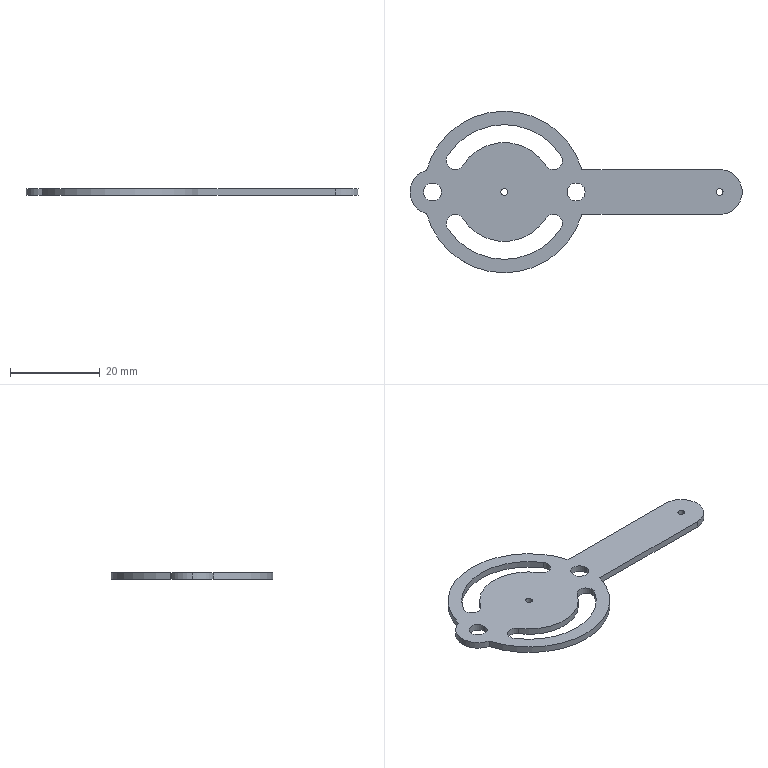Part | SolidWorks | features Extrusion 1 | 1 solid | 27 faces | box 74 x 36 x 1.5 mm | volume 1679 mm3 | cylinder 23 | plane 4 | commonest cylinder face diameters 4 x10 1.5 x4 10 x3 22 x2 30 x2 36 x2
STEP:
#1=CARTESIAN_POINT('',(47.25,0.,1.5));
#2=VERTEX_POINT('',#1);
#3=CARTESIAN_POINT('',(48.75,0.,1.5));
#4=VERTEX_POINT('',#3);
#5=CARTESIAN_POINT('',(48.,0.,1.5));
#6=DIRECTION('',(0.,0.,1.));
#7=DIRECTION('',(1.,0.,0.));
#8=AXIS2_PLACEMENT_3D('',#5,#6,#7);
#9=CIRCLE('',#8,0.75);
#10=EDGE_CURVE('',#2,#4,#9,.T.);
#11=ORIENTED_EDGE('',*,*,#10,.T.);
#12=CARTESIAN_POINT('',(48.75,0.,0.));
#13=VERTEX_POINT('',#12);
#14=CARTESIAN_POINT('',(48.75,0.,1.5));
#15=DIRECTION('',(0.,0.,-1.));
#16=VECTOR('',#15,1000.);
#17=LINE('',#14,#16);
#18=EDGE_CURVE('',#4,#13,#17,.T.);
#19=ORIENTED_EDGE('',*,*,#18,.T.);
#20=CARTESIAN_POINT('',(47.25,0.,0.));
#21=VERTEX_POINT('',#20);
#22=CARTESIAN_POINT('',(48.,0.,0.));
#23=DIRECTION('',(0.,0.,1.));
#24=DIRECTION('',(1.,0.,0.));
#25=AXIS2_PLACEMENT_3D('',#22,#23,#24);
#26=CIRCLE('',#25,0.75);
#27=EDGE_CURVE('',#21,#13,#26,.T.);
#28=ORIENTED_EDGE('',*,*,#27,.F.);
#29=CARTESIAN_POINT('',(47.25,0.,1.5));
#30=DIRECTION('',(0.,0.,-1.));
#31=VECTOR('',#30,1000.);
#32=LINE('',#29,#31);
#33=EDGE_CURVE('',#2,#21,#32,.T.);
#34=ORIENTED_EDGE('',*,*,#33,.F.);
#35=EDGE_LOOP('',(#11,#19,#28,#34));
#36=FACE_OUTER_BOUND('',#35,.T.);
#37=CARTESIAN_POINT('',(48.,0.,1.5));
#38=DIRECTION('',(0.,0.,-1.));
#39=DIRECTION('',(-1.,0.,0.));
#40=AXIS2_PLACEMENT_3D('',#37,#38,#39);
#41=CYLINDRICAL_SURFACE('',#40,0.75);
#42=ADVANCED_FACE('',(#36),#41,.F.);
#43=CARTESIAN_POINT('',(-18.,0.,1.5));
#44=VERTEX_POINT('',#43);
#45=CARTESIAN_POINT('',(-14.,0.,1.5));
#46=VERTEX_POINT('',#45);
#47=CARTESIAN_POINT('',(-16.,0.,1.5));
#48=DIRECTION('',(0.,0.,1.));
#49=DIRECTION('',(1.,0.,0.));
#50=AXIS2_PLACEMENT_3D('',#47,#48,#49);
#51=CIRCLE('',#50,2.);
#52=EDGE_CURVE('',#44,#46,#51,.T.);
#53=ORIENTED_EDGE('',*,*,#52,.T.);
#54=CARTESIAN_POINT('',(-14.,0.,0.));
#55=VERTEX_POINT('',#54);
#56=CARTESIAN_POINT('',(-14.,0.,1.5));
#57=DIRECTION('',(0.,0.,-1.));
#58=VECTOR('',#57,1000.);
#59=LINE('',#56,#58);
#60=EDGE_CURVE('',#46,#55,#59,.T.);
#61=ORIENTED_EDGE('',*,*,#60,.T.);
#62=CARTESIAN_POINT('',(-18.,0.,0.));
#63=VERTEX_POINT('',#62);
#64=CARTESIAN_POINT('',(-16.,0.,0.));
#65=DIRECTION('',(0.,0.,1.));
#66=DIRECTION('',(1.,0.,0.));
#67=AXIS2_PLACEMENT_3D('',#64,#65,#66);
#68=CIRCLE('',#67,2.);
#69=EDGE_CURVE('',#63,#55,#68,.T.);
#70=ORIENTED_EDGE('',*,*,#69,.F.);
#71=CARTESIAN_POINT('',(-18.,0.,1.5));
#72=DIRECTION('',(0.,0.,-1.));
#73=VECTOR('',#72,1000.);
#74=LINE('',#71,#73);
#75=EDGE_CURVE('',#44,#63,#74,.T.);
#76=ORIENTED_EDGE('',*,*,#75,.F.);
#77=EDGE_LOOP('',(#53,#61,#70,#76));
#78=FACE_OUTER_BOUND('',#77,.T.);
#79=CARTESIAN_POINT('',(-16.,0.,1.5));
#80=DIRECTION('',(0.,0.,-1.));
#81=DIRECTION('',(-1.,0.,0.));
#82=AXIS2_PLACEMENT_3D('',#79,#80,#81);
#83=CYLINDRICAL_SURFACE('',#82,2.);
#84=ADVANCED_FACE('',(#78),#83,.F.);
#85=CARTESIAN_POINT('',(14.,0.,1.5));
#86=VERTEX_POINT('',#85);
#87=CARTESIAN_POINT('',(18.,0.,1.5));
#88=VERTEX_POINT('',#87);
#89=CARTESIAN_POINT('',(16.,0.,1.5));
#90=DIRECTION('',(0.,0.,1.));
#91=DIRECTION('',(1.,0.,0.));
#92=AXIS2_PLACEMENT_3D('',#89,#90,#91);
#93=CIRCLE('',#92,2.);
#94=EDGE_CURVE('',#86,#88,#93,.T.);
#95=ORIENTED_EDGE('',*,*,#94,.T.);
#96=CARTESIAN_POINT('',(18.,0.,0.));
#97=VERTEX_POINT('',#96);
#98=CARTESIAN_POINT('',(18.,0.,1.5));
#99=DIRECTION('',(0.,0.,-1.));
#100=VECTOR('',#99,1000.);
#101=LINE('',#98,#100);
#102=EDGE_CURVE('',#88,#97,#101,.T.);
#103=ORIENTED_EDGE('',*,*,#102,.T.);
#104=CARTESIAN_POINT('',(14.,0.,0.));
#105=VERTEX_POINT('',#104);
#106=CARTESIAN_POINT('',(16.,0.,0.));
#107=DIRECTION('',(0.,0.,1.));
#108=DIRECTION('',(1.,0.,0.));
#109=AXIS2_PLACEMENT_3D('',#106,#107,#108);
#110=CIRCLE('',#109,2.);
#111=EDGE_CURVE('',#105,#97,#110,.T.);
#112=ORIENTED_EDGE('',*,*,#111,.F.);
#113=CARTESIAN_POINT('',(14.,0.,1.5));
#114=DIRECTION('',(0.,0.,-1.));
#115=VECTOR('',#114,1000.);
#116=LINE('',#113,#115);
#117=EDGE_CURVE('',#86,#105,#116,.T.);
#118=ORIENTED_EDGE('',*,*,#117,.F.);
#119=EDGE_LOOP('',(#95,#103,#112,#118));
#120=FACE_OUTER_BOUND('',#119,.T.);
#121=CARTESIAN_POINT('',(16.,0.,1.5));
#122=DIRECTION('',(0.,0.,-1.));
#123=DIRECTION('',(-1.,0.,0.));
#124=AXIS2_PLACEMENT_3D('',#121,#122,#123);
#125=CYLINDRICAL_SURFACE('',#124,2.);
#126=ADVANCED_FACE('',(#120),#125,.F.);
#127=CARTESIAN_POINT('',(-9.269,-5.923,1.5));
#128=VERTEX_POINT('',#127);
#129=CARTESIAN_POINT('',(-12.954,-7.,1.5));
#130=VERTEX_POINT('',#129);
#131=CARTESIAN_POINT('',(-10.954,-7.,1.5));
#132=DIRECTION('',(0.,0.,1.));
#133=DIRECTION('',(1.,0.,0.));
#134=AXIS2_PLACEMENT_3D('',#131,#132,#133);
#135=CIRCLE('',#134,2.);
#136=EDGE_CURVE('',#128,#130,#135,.T.);
#137=ORIENTED_EDGE('',*,*,#136,.T.);
#138=CARTESIAN_POINT('',(-12.954,-7.,0.));
#139=VERTEX_POINT('',#138);
#140=CARTESIAN_POINT('',(-12.954,-7.,1.5));
#141=DIRECTION('',(0.,0.,-1.));
#142=VECTOR('',#141,1000.);
#143=LINE('',#140,#142);
#144=EDGE_CURVE('',#130,#139,#143,.T.);
#145=ORIENTED_EDGE('',*,*,#144,.T.);
#146=CARTESIAN_POINT('',(-9.269,-5.923,0.));
#147=VERTEX_POINT('',#146);
#148=CARTESIAN_POINT('',(-10.954,-7.,0.));
#149=DIRECTION('',(0.,0.,1.));
#150=DIRECTION('',(1.,0.,0.));
#151=AXIS2_PLACEMENT_3D('',#148,#149,#150);
#152=CIRCLE('',#151,2.);
#153=EDGE_CURVE('',#147,#139,#152,.T.);
#154=ORIENTED_EDGE('',*,*,#153,.F.);
#155=CARTESIAN_POINT('',(-9.269,-5.923,1.5));
#156=DIRECTION('',(0.,0.,-1.));
#157=VECTOR('',#156,1000.);
#158=LINE('',#155,#157);
#159=EDGE_CURVE('',#128,#147,#158,.T.);
#160=ORIENTED_EDGE('',*,*,#159,.F.);
#161=EDGE_LOOP('',(#137,#145,#154,#160));
#162=FACE_OUTER_BOUND('',#161,.T.);
#163=CARTESIAN_POINT('',(-10.954,-7.,1.5));
#164=DIRECTION('',(0.,0.,-1.));
#165=DIRECTION('',(-1.,0.,0.));
#166=AXIS2_PLACEMENT_3D('',#163,#164,#165);
#167=CYLINDRICAL_SURFACE('',#166,2.);
#168=ADVANCED_FACE('',(#162),#167,.F.);
#169=CARTESIAN_POINT('',(-0.75,0.,1.5));
#170=VERTEX_POINT('',#169);
#171=CARTESIAN_POINT('',(0.75,0.,1.5));
#172=VERTEX_POINT('',#171);
#173=CARTESIAN_POINT('',(0.,0.,1.5));
#174=DIRECTION('',(0.,0.,1.));
#175=DIRECTION('',(1.,0.,0.));
#176=AXIS2_PLACEMENT_3D('',#173,#174,#175);
#177=CIRCLE('',#176,0.75);
#178=EDGE_CURVE('',#170,#172,#177,.T.);
#179=ORIENTED_EDGE('',*,*,#178,.T.);
#180=CARTESIAN_POINT('',(0.75,0.,0.));
#181=VERTEX_POINT('',#180);
#182=CARTESIAN_POINT('',(0.75,0.,1.5));
#183=DIRECTION('',(0.,0.,-1.));
#184=VECTOR('',#183,1000.);
#185=LINE('',#182,#184);
#186=EDGE_CURVE('',#172,#181,#185,.T.);
#187=ORIENTED_EDGE('',*,*,#186,.T.);
#188=CARTESIAN_POINT('',(-0.75,0.,0.));
#189=VERTEX_POINT('',#188);
#190=CARTESIAN_POINT('',(0.,0.,0.));
#191=DIRECTION('',(0.,0.,1.));
#192=DIRECTION('',(1.,0.,0.));
#193=AXIS2_PLACEMENT_3D('',#190,#191,#192);
#194=CIRCLE('',#193,0.75);
#195=EDGE_CURVE('',#189,#181,#194,.T.);
#196=ORIENTED_EDGE('',*,*,#195,.F.);
#197=CARTESIAN_POINT('',(-0.75,0.,1.5));
#198=DIRECTION('',(0.,0.,-1.));
#199=VECTOR('',#198,1000.);
#200=LINE('',#197,#199);
#201=EDGE_CURVE('',#170,#189,#200,.T.);
#202=ORIENTED_EDGE('',*,*,#201,.F.);
#203=EDGE_LOOP('',(#179,#187,#196,#202));
#204=FACE_OUTER_BOUND('',#203,.T.);
#205=CARTESIAN_POINT('',(0.,0.,1.5));
#206=DIRECTION('',(0.,0.,-1.));
#207=DIRECTION('',(-1.,0.,0.));
#208=AXIS2_PLACEMENT_3D('',#205,#206,#207);
#209=CYLINDRICAL_SURFACE('',#208,0.75);
#210=ADVANCED_FACE('',(#204),#209,.F.);
#211=CARTESIAN_POINT('',(-12.64,8.077,1.5));
#212=VERTEX_POINT('',#211);
#213=CARTESIAN_POINT('',(-12.954,7.,1.5));
#214=VERTEX_POINT('',#213);
#215=CARTESIAN_POINT('',(-10.954,7.,1.5));
#216=DIRECTION('',(0.,0.,1.));
#217=DIRECTION('',(1.,0.,0.));
#218=AXIS2_PLACEMENT_3D('',#215,#216,#217);
#219=CIRCLE('',#218,2.);
#220=EDGE_CURVE('',#212,#214,#219,.T.);
#221=ORIENTED_EDGE('',*,*,#220,.T.);
#222=CARTESIAN_POINT('',(-12.954,7.,0.));
#223=VERTEX_POINT('',#222);
#224=CARTESIAN_POINT('',(-12.954,7.,1.5));
#225=DIRECTION('',(0.,0.,-1.));
#226=VECTOR('',#225,1000.);
#227=LINE('',#224,#226);
#228=EDGE_CURVE('',#214,#223,#227,.T.);
#229=ORIENTED_EDGE('',*,*,#228,.T.);
#230=CARTESIAN_POINT('',(-12.64,8.077,0.));
#231=VERTEX_POINT('',#230);
#232=CARTESIAN_POINT('',(-10.954,7.,0.));
#233=DIRECTION('',(0.,0.,1.));
#234=DIRECTION('',(1.,0.,0.));
#235=AXIS2_PLACEMENT_3D('',#232,#233,#234);
#236=CIRCLE('',#235,2.);
#237=EDGE_CURVE('',#231,#223,#236,.T.);
#238=ORIENTED_EDGE('',*,*,#237,.F.);
#239=CARTESIAN_POINT('',(-12.64,8.077,1.5));
#240=DIRECTION('',(0.,0.,-1.));
#241=VECTOR('',#240,1000.);
#242=LINE('',#239,#241);
#243=EDGE_CURVE('',#212,#231,#242,.T.);
#244=ORIENTED_EDGE('',*,*,#243,.F.);
#245=EDGE_LOOP('',(#221,#229,#238,#244));
#246=FACE_OUTER_BOUND('',#245,.T.);
#247=CARTESIAN_POINT('',(-10.954,7.,1.5));
#248=DIRECTION('',(0.,0.,-1.));
#249=DIRECTION('',(-1.,0.,0.));
#250=AXIS2_PLACEMENT_3D('',#247,#248,#249);
#251=CYLINDRICAL_SURFACE('',#250,2.);
#252=ADVANCED_FACE('',(#246),#251,.F.);
#253=CARTESIAN_POINT('',(-21.,0.,1.5));
#254=VERTEX_POINT('',#253);
#255=CARTESIAN_POINT('',(-17.344,-4.816,1.5));
#256=VERTEX_POINT('',#255);
#257=CARTESIAN_POINT('',(-16.,0.,1.5));
#258=DIRECTION('',(0.,0.,1.));
#259=DIRECTION('',(1.,0.,0.));
#260=AXIS2_PLACEMENT_3D('',#257,#258,#259);
#261=CIRCLE('',#260,5.);
#262=EDGE_CURVE('',#254,#256,#261,.T.);
#263=ORIENTED_EDGE('',*,*,#262,.F.);
#264=CARTESIAN_POINT('',(-21.,0.,0.));
#265=VERTEX_POINT('',#264);
#266=CARTESIAN_POINT('',(-21.,0.,1.5));
#267=DIRECTION('',(0.,0.,-1.));
#268=VECTOR('',#267,1000.);
#269=LINE('',#266,#268);
#270=EDGE_CURVE('',#254,#265,#269,.T.);
#271=ORIENTED_EDGE('',*,*,#270,.T.);
#272=CARTESIAN_POINT('',(-17.344,-4.816,0.));
#273=VERTEX_POINT('',#272);
#274=CARTESIAN_POINT('',(-16.,0.,0.));
#275=DIRECTION('',(0.,0.,1.));
#276=DIRECTION('',(1.,0.,0.));
#277=AXIS2_PLACEMENT_3D('',#274,#275,#276);
#278=CIRCLE('',#277,5.);
#279=EDGE_CURVE('',#265,#273,#278,.T.);
#280=ORIENTED_EDGE('',*,*,#279,.T.);
#281=CARTESIAN_POINT('',(-17.344,-4.816,1.5));
#282=DIRECTION('',(0.,0.,-1.));
#283=VECTOR('',#282,1000.);
#284=LINE('',#281,#283);
#285=EDGE_CURVE('',#256,#273,#284,.T.);
#286=ORIENTED_EDGE('',*,*,#285,.F.);
#287=EDGE_LOOP('',(#263,#271,#280,#286));
#288=FACE_OUTER_BOUND('',#287,.T.);
#289=CARTESIAN_POINT('',(-16.,0.,1.5));
#290=DIRECTION('',(0.,0.,-1.));
#291=DIRECTION('',(-1.,0.,0.));
#292=AXIS2_PLACEMENT_3D('',#289,#290,#291);
#293=CYLINDRICAL_SURFACE('',#292,5.);
#294=ADVANCED_FACE('',(#288),#293,.T.);
#295=ORIENTED_EDGE('',*,*,#52,.F.);
#296=CARTESIAN_POINT('',(-16.,0.,1.5));
#297=DIRECTION('',(0.,0.,1.));
#298=DIRECTION('',(1.,0.,0.));
#299=AXIS2_PLACEMENT_3D('',#296,#297,#298);
#300=CIRCLE('',#299,2.);
#301=EDGE_CURVE('',#46,#44,#300,.T.);
#302=ORIENTED_EDGE('',*,*,#301,.F.);
#303=EDGE_LOOP('',(#295,#302));
#304=FACE_BOUND('',#303,.T.);
#305=ORIENTED_EDGE('',*,*,#136,.F.);
#306=CARTESIAN_POINT('',(9.269,-5.923,1.5));
#307=VERTEX_POINT('',#306);
#308=CARTESIAN_POINT('',(0.,0.,1.5));
#309=DIRECTION('',(0.,0.,-1.));
#310=DIRECTION('',(1.,0.,0.));
#311=AXIS2_PLACEMENT_3D('',#308,#309,#310);
#312=CIRCLE('',#311,11.);
#313=EDGE_CURVE('',#307,#128,#312,.T.);
#314=ORIENTED_EDGE('',*,*,#313,.F.);
#315=CARTESIAN_POINT('',(12.64,-8.077,1.5));
#316=VERTEX_POINT('',#315);
#317=CARTESIAN_POINT('',(10.954,-7.,1.5));
#318=DIRECTION('',(0.,0.,1.));
#319=DIRECTION('',(1.,0.,0.));
#320=AXIS2_PLACEMENT_3D('',#317,#318,#319);
#321=CIRCLE('',#320,2.);
#322=EDGE_CURVE('',#316,#307,#321,.T.);
#323=ORIENTED_EDGE('',*,*,#322,.F.);
#324=CARTESIAN_POINT('',(-12.64,-8.077,1.5));
#325=VERTEX_POINT('',#324);
#326=CARTESIAN_POINT('',(0.,0.,1.5));
#327=DIRECTION('',(0.,0.,1.));
#328=DIRECTION('',(1.,0.,0.));
#329=AXIS2_PLACEMENT_3D('',#326,#327,#328);
#330=CIRCLE('',#329,15.);
#331=EDGE_CURVE('',#325,#316,#330,.T.);
#332=ORIENTED_EDGE('',*,*,#331,.F.);
#333=CARTESIAN_POINT('',(-10.954,-7.,1.5));
#334=DIRECTION('',(0.,0.,1.));
#335=DIRECTION('',(1.,0.,0.));
#336=AXIS2_PLACEMENT_3D('',#333,#334,#335);
#337=CIRCLE('',#336,2.);
#338=EDGE_CURVE('',#130,#325,#337,.T.);
#339=ORIENTED_EDGE('',*,*,#338,.F.);
#340=EDGE_LOOP('',(#305,#314,#323,#332,#339));
#341=FACE_BOUND('',#340,.T.);
#342=ORIENTED_EDGE('',*,*,#178,.F.);
#343=CARTESIAN_POINT('',(0.,0.,1.5));
#344=DIRECTION('',(0.,0.,1.));
#345=DIRECTION('',(1.,0.,0.));
#346=AXIS2_PLACEMENT_3D('',#343,#344,#345);
#347=CIRCLE('',#346,0.75);
#348=EDGE_CURVE('',#172,#170,#347,.T.);
#349=ORIENTED_EDGE('',*,*,#348,.F.);
#350=EDGE_LOOP('',(#342,#349));
#351=FACE_BOUND('',#350,.T.);
#352=CARTESIAN_POINT('',(-17.344,4.816,1.5));
#353=VERTEX_POINT('',#352);
#354=CARTESIAN_POINT('',(-16.,0.,1.5));
#355=DIRECTION('',(0.,0.,1.));
#356=DIRECTION('',(1.,0.,0.));
#357=AXIS2_PLACEMENT_3D('',#354,#355,#356);
#358=CIRCLE('',#357,5.);
#359=EDGE_CURVE('',#353,#254,#358,.T.);
#360=ORIENTED_EDGE('',*,*,#359,.T.);
#361=ORIENTED_EDGE('',*,*,#262,.T.);
#362=CARTESIAN_POINT('',(17.292,-5.,1.5));
#363=VERTEX_POINT('',#362);
#364=CARTESIAN_POINT('',(0.,0.,1.5));
#365=DIRECTION('',(0.,0.,1.));
#366=DIRECTION('',(1.,0.,0.));
#367=AXIS2_PLACEMENT_3D('',#364,#365,#366);
#368=CIRCLE('',#367,18.);
#369=EDGE_CURVE('',#256,#363,#368,.T.);
#370=ORIENTED_EDGE('',*,*,#369,.T.);
#371=CARTESIAN_POINT('',(48.,-5.,1.5));
#372=VERTEX_POINT('',#371);
#373=CARTESIAN_POINT('',(48.,-5.,1.5));
#374=DIRECTION('',(1.,0.,0.));
#375=VECTOR('',#374,1000.);
#376=LINE('',#373,#375);
#377=EDGE_CURVE('',#363,#372,#376,.T.);
#378=ORIENTED_EDGE('',*,*,#377,.T.);
#379=CARTESIAN_POINT('',(48.,5.,1.5));
#380=VERTEX_POINT('',#379);
#381=CARTESIAN_POINT('',(48.,0.,1.5));
#382=DIRECTION('',(0.,0.,1.));
#383=DIRECTION('',(-1.,0.,0.));
#384=AXIS2_PLACEMENT_3D('',#381,#382,#383);
#385=CIRCLE('',#384,5.);
#386=EDGE_CURVE('',#372,#380,#385,.T.);
#387=ORIENTED_EDGE('',*,*,#386,.T.);
#388=CARTESIAN_POINT('',(17.292,5.,1.5));
#389=VERTEX_POINT('',#388);
#390=CARTESIAN_POINT('',(48.,5.,1.5));
#391=DIRECTION('',(-1.,0.,0.));
#392=VECTOR('',#391,1000.);
#393=LINE('',#390,#392);
#394=EDGE_CURVE('',#380,#389,#393,.T.);
#395=ORIENTED_EDGE('',*,*,#394,.T.);
#396=CARTESIAN_POINT('',(0.,0.,1.5));
#397=DIRECTION('',(0.,0.,1.));
#398=DIRECTION('',(1.,0.,0.));
#399=AXIS2_PLACEMENT_3D('',#396,#397,#398);
#400=CIRCLE('',#399,18.);
#401=EDGE_CURVE('',#389,#353,#400,.T.);
#402=ORIENTED_EDGE('',*,*,#401,.T.);
#403=EDGE_LOOP('',(#360,#361,#370,#378,#387,#395,#402));
#404=FACE_OUTER_BOUND('',#403,.T.);
#405=ORIENTED_EDGE('',*,*,#220,.F.);
#406=CARTESIAN_POINT('',(12.64,8.077,1.5));
#407=VERTEX_POINT('',#406);
#408=CARTESIAN_POINT('',(0.,0.,1.5));
#409=DIRECTION('',(0.,0.,1.));
#410=DIRECTION('',(1.,0.,0.));
#411=AXIS2_PLACEMENT_3D('',#408,#409,#410);
#412=CIRCLE('',#411,15.);
#413=EDGE_CURVE('',#407,#212,#412,.T.);
#414=ORIENTED_EDGE('',*,*,#413,.F.);
#415=CARTESIAN_POINT('',(9.269,5.923,1.5));
#416=VERTEX_POINT('',#415);
#417=CARTESIAN_POINT('',(10.954,7.,1.5));
#418=DIRECTION('',(0.,0.,1.));
#419=DIRECTION('',(1.,0.,0.));
#420=AXIS2_PLACEMENT_3D('',#417,#418,#419);
#421=CIRCLE('',#420,2.);
#422=EDGE_CURVE('',#416,#407,#421,.T.);
#423=ORIENTED_EDGE('',*,*,#422,.F.);
#424=CARTESIAN_POINT('',(-9.269,5.923,1.5));
#425=VERTEX_POINT('',#424);
#426=CARTESIAN_POINT('',(0.,0.,1.5));
#427=DIRECTION('',(0.,0.,-1.));
#428=DIRECTION('',(1.,0.,0.));
#429=AXIS2_PLACEMENT_3D('',#426,#427,#428);
#430=CIRCLE('',#429,11.);
#431=EDGE_CURVE('',#425,#416,#430,.T.);
#432=ORIENTED_EDGE('',*,*,#431,.F.);
#433=CARTESIAN_POINT('',(-10.954,7.,1.5));
#434=DIRECTION('',(0.,0.,1.));
#435=DIRECTION('',(1.,0.,0.));
#436=AXIS2_PLACEMENT_3D('',#433,#434,#435);
#437=CIRCLE('',#436,2.);
#438=EDGE_CURVE('',#214,#425,#437,.T.);
#439=ORIENTED_EDGE('',*,*,#438,.F.);
#440=EDGE_LOOP('',(#405,#414,#423,#432,#439));
#441=FACE_BOUND('',#440,.T.);
#442=ORIENTED_EDGE('',*,*,#94,.F.);
#443=CARTESIAN_POINT('',(16.,0.,1.5));
#444=DIRECTION('',(0.,0.,1.));
#445=DIRECTION('',(1.,0.,0.));
#446=AXIS2_PLACEMENT_3D('',#443,#444,#445);
#447=CIRCLE('',#446,2.);
#448=EDGE_CURVE('',#88,#86,#447,.T.);
#449=ORIENTED_EDGE('',*,*,#448,.F.);
#450=EDGE_LOOP('',(#442,#449));
#451=FACE_BOUND('',#450,.T.);
#452=ORIENTED_EDGE('',*,*,#10,.F.);
#453=CARTESIAN_POINT('',(48.,0.,1.5));
#454=DIRECTION('',(0.,0.,1.));
#455=DIRECTION('',(1.,0.,0.));
#456=AXIS2_PLACEMENT_3D('',#453,#454,#455);
#457=CIRCLE('',#456,0.75);
#458=EDGE_CURVE('',#4,#2,#457,.T.);
#459=ORIENTED_EDGE('',*,*,#458,.F.);
#460=EDGE_LOOP('',(#452,#459));
#461=FACE_BOUND('',#460,.T.);
#462=CARTESIAN_POINT('',(-16.,0.,1.5));
#463=DIRECTION('',(0.,0.,1.));
#464=DIRECTION('',(1.,0.,0.));
#465=AXIS2_PLACEMENT_3D('',#462,#463,#464);
#466=PLANE('',#465);
#467=ADVANCED_FACE('',(#304,#341,#351,#404,#441,#451,#461),#466,.T.);
#468=ORIENTED_EDGE('',*,*,#195,.T.);
#469=CARTESIAN_POINT('',(0.,0.,0.));
#470=DIRECTION('',(0.,0.,1.));
#471=DIRECTION('',(1.,0.,0.));
#472=AXIS2_PLACEMENT_3D('',#469,#470,#471);
#473=CIRCLE('',#472,0.75);
#474=EDGE_CURVE('',#181,#189,#473,.T.);
#475=ORIENTED_EDGE('',*,*,#474,.T.);
#476=EDGE_LOOP('',(#468,#475));
#477=FACE_BOUND('',#476,.T.);
#478=CARTESIAN_POINT('',(12.64,8.077,0.));
#479=VERTEX_POINT('',#478);
#480=CARTESIAN_POINT('',(0.,0.,0.));
#481=DIRECTION('',(0.,0.,1.));
#482=DIRECTION('',(1.,0.,0.));
#483=AXIS2_PLACEMENT_3D('',#480,#481,#482);
#484=CIRCLE('',#483,15.);
#485=EDGE_CURVE('',#479,#231,#484,.T.);
#486=ORIENTED_EDGE('',*,*,#485,.T.);
#487=ORIENTED_EDGE('',*,*,#237,.T.);
#488=CARTESIAN_POINT('',(-9.269,5.923,0.));
#489=VERTEX_POINT('',#488);
#490=CARTESIAN_POINT('',(-10.954,7.,0.));
#491=DIRECTION('',(0.,0.,1.));
#492=DIRECTION('',(1.,0.,0.));
#493=AXIS2_PLACEMENT_3D('',#490,#491,#492);
#494=CIRCLE('',#493,2.);
#495=EDGE_CURVE('',#223,#489,#494,.T.);
#496=ORIENTED_EDGE('',*,*,#495,.T.);
#497=CARTESIAN_POINT('',(9.269,5.923,0.));
#498=VERTEX_POINT('',#497);
#499=CARTESIAN_POINT('',(0.,0.,0.));
#500=DIRECTION('',(0.,0.,-1.));
#501=DIRECTION('',(1.,0.,0.));
#502=AXIS2_PLACEMENT_3D('',#499,#500,#501);
#503=CIRCLE('',#502,11.);
#504=EDGE_CURVE('',#489,#498,#503,.T.);
#505=ORIENTED_EDGE('',*,*,#504,.T.);
#506=CARTESIAN_POINT('',(10.954,7.,0.));
#507=DIRECTION('',(0.,0.,1.));
#508=DIRECTION('',(1.,0.,0.));
#509=AXIS2_PLACEMENT_3D('',#506,#507,#508);
#510=CIRCLE('',#509,2.);
#511=EDGE_CURVE('',#498,#479,#510,.T.);
#512=ORIENTED_EDGE('',*,*,#511,.T.);
#513=EDGE_LOOP('',(#486,#487,#496,#505,#512));
#514=FACE_BOUND('',#513,.T.);
#515=CARTESIAN_POINT('',(-17.344,4.816,0.));
#516=VERTEX_POINT('',#515);
#517=CARTESIAN_POINT('',(-16.,0.,0.));
#518=DIRECTION('',(0.,0.,1.));
#519=DIRECTION('',(1.,0.,0.));
#520=AXIS2_PLACEMENT_3D('',#517,#518,#519);
#521=CIRCLE('',#520,5.);
#522=EDGE_CURVE('',#516,#265,#521,.T.);
#523=ORIENTED_EDGE('',*,*,#522,.F.);
#524=CARTESIAN_POINT('',(17.292,5.,0.));
#525=VERTEX_POINT('',#524);
#526=CARTESIAN_POINT('',(0.,0.,0.));
#527=DIRECTION('',(0.,0.,1.));
#528=DIRECTION('',(1.,0.,0.));
#529=AXIS2_PLACEMENT_3D('',#526,#527,#528);
#530=CIRCLE('',#529,18.);
#531=EDGE_CURVE('',#525,#516,#530,.T.);
#532=ORIENTED_EDGE('',*,*,#531,.F.);
#533=CARTESIAN_POINT('',(48.,5.,0.));
#534=VERTEX_POINT('',#533);
#535=CARTESIAN_POINT('',(48.,5.,0.));
#536=DIRECTION('',(-1.,0.,0.));
#537=VECTOR('',#536,1000.);
#538=LINE('',#535,#537);
#539=EDGE_CURVE('',#534,#525,#538,.T.);
#540=ORIENTED_EDGE('',*,*,#539,.F.);
#541=CARTESIAN_POINT('',(48.,-5.,0.));
#542=VERTEX_POINT('',#541);
#543=CARTESIAN_POINT('',(48.,0.,0.));
#544=DIRECTION('',(0.,0.,1.));
#545=DIRECTION('',(-1.,0.,0.));
#546=AXIS2_PLACEMENT_3D('',#543,#544,#545);
#547=CIRCLE('',#546,5.);
#548=EDGE_CURVE('',#542,#534,#547,.T.);
#549=ORIENTED_EDGE('',*,*,#548,.F.);
#550=CARTESIAN_POINT('',(17.292,-5.,0.));
#551=VERTEX_POINT('',#550);
#552=CARTESIAN_POINT('',(48.,-5.,0.));
#553=DIRECTION('',(1.,0.,0.));
#554=VECTOR('',#553,1000.);
#555=LINE('',#552,#554);
#556=EDGE_CURVE('',#551,#542,#555,.T.);
#557=ORIENTED_EDGE('',*,*,#556,.F.);
#558=CARTESIAN_POINT('',(0.,0.,0.));
#559=DIRECTION('',(0.,0.,1.));
#560=DIRECTION('',(1.,0.,0.));
#561=AXIS2_PLACEMENT_3D('',#558,#559,#560);
#562=CIRCLE('',#561,18.);
#563=EDGE_CURVE('',#273,#551,#562,.T.);
#564=ORIENTED_EDGE('',*,*,#563,.F.);
#565=ORIENTED_EDGE('',*,*,#279,.F.);
#566=EDGE_LOOP('',(#523,#532,#540,#549,#557,#564,#565));
#567=FACE_OUTER_BOUND('',#566,.T.);
#568=CARTESIAN_POINT('',(9.269,-5.923,0.));
#569=VERTEX_POINT('',#568);
#570=CARTESIAN_POINT('',(0.,0.,0.));
#571=DIRECTION('',(0.,0.,-1.));
#572=DIRECTION('',(1.,0.,0.));
#573=AXIS2_PLACEMENT_3D('',#570,#571,#572);
#574=CIRCLE('',#573,11.);
#575=EDGE_CURVE('',#569,#147,#574,.T.);
#576=ORIENTED_EDGE('',*,*,#575,.T.);
#577=ORIENTED_EDGE('',*,*,#153,.T.);
#578=CARTESIAN_POINT('',(-12.64,-8.077,0.));
#579=VERTEX_POINT('',#578);
#580=CARTESIAN_POINT('',(-10.954,-7.,0.));
#581=DIRECTION('',(0.,0.,1.));
#582=DIRECTION('',(1.,0.,0.));
#583=AXIS2_PLACEMENT_3D('',#580,#581,#582);
#584=CIRCLE('',#583,2.);
#585=EDGE_CURVE('',#139,#579,#584,.T.);
#586=ORIENTED_EDGE('',*,*,#585,.T.);
#587=CARTESIAN_POINT('',(12.64,-8.077,0.));
#588=VERTEX_POINT('',#587);
#589=CARTESIAN_POINT('',(0.,0.,0.));
#590=DIRECTION('',(0.,0.,1.));
#591=DIRECTION('',(1.,0.,0.));
#592=AXIS2_PLACEMENT_3D('',#589,#590,#591);
#593=CIRCLE('',#592,15.);
#594=EDGE_CURVE('',#579,#588,#593,.T.);
#595=ORIENTED_EDGE('',*,*,#594,.T.);
#596=CARTESIAN_POINT('',(10.954,-7.,0.));
#597=DIRECTION('',(0.,0.,1.));
#598=DIRECTION('',(1.,0.,0.));
#599=AXIS2_PLACEMENT_3D('',#596,#597,#598);
#600=CIRCLE('',#599,2.);
#601=EDGE_CURVE('',#588,#569,#600,.T.);
#602=ORIENTED_EDGE('',*,*,#601,.T.);
#603=EDGE_LOOP('',(#576,#577,#586,#595,#602));
#604=FACE_BOUND('',#603,.T.);
#605=ORIENTED_EDGE('',*,*,#111,.T.);
#606=CARTESIAN_POINT('',(16.,0.,0.));
#607=DIRECTION('',(0.,0.,1.));
#608=DIRECTION('',(1.,0.,0.));
#609=AXIS2_PLACEMENT_3D('',#606,#607,#608);
#610=CIRCLE('',#609,2.);
#611=EDGE_CURVE('',#97,#105,#610,.T.);
#612=ORIENTED_EDGE('',*,*,#611,.T.);
#613=EDGE_LOOP('',(#605,#612));
#614=FACE_BOUND('',#613,.T.);
#615=ORIENTED_EDGE('',*,*,#69,.T.);
#616=CARTESIAN_POINT('',(-16.,0.,0.));
#617=DIRECTION('',(0.,0.,1.));
#618=DIRECTION('',(1.,0.,0.));
#619=AXIS2_PLACEMENT_3D('',#616,#617,#618);
#620=CIRCLE('',#619,2.);
#621=EDGE_CURVE('',#55,#63,#620,.T.);
#622=ORIENTED_EDGE('',*,*,#621,.T.);
#623=EDGE_LOOP('',(#615,#622));
#624=FACE_BOUND('',#623,.T.);
#625=ORIENTED_EDGE('',*,*,#27,.T.);
#626=CARTESIAN_POINT('',(48.,0.,0.));
#627=DIRECTION('',(0.,0.,1.));
#628=DIRECTION('',(1.,0.,0.));
#629=AXIS2_PLACEMENT_3D('',#626,#627,#628);
#630=CIRCLE('',#629,0.75);
#631=EDGE_CURVE('',#13,#21,#630,.T.);
#632=ORIENTED_EDGE('',*,*,#631,.T.);
#633=EDGE_LOOP('',(#625,#632));
#634=FACE_BOUND('',#633,.T.);
#635=CARTESIAN_POINT('',(-16.,0.,0.));
#636=DIRECTION('',(0.,0.,1.));
#637=DIRECTION('',(1.,0.,0.));
#638=AXIS2_PLACEMENT_3D('',#635,#636,#637);
#639=PLANE('',#638);
#640=ADVANCED_FACE('',(#477,#514,#567,#604,#614,#624,#634),#639,.F.);
#641=ORIENTED_EDGE('',*,*,#270,.F.);
#642=ORIENTED_EDGE('',*,*,#359,.F.);
#643=CARTESIAN_POINT('',(-17.344,4.816,1.5));
#644=DIRECTION('',(0.,0.,-1.));
#645=VECTOR('',#644,1000.);
#646=LINE('',#643,#645);
#647=EDGE_CURVE('',#353,#516,#646,.T.);
#648=ORIENTED_EDGE('',*,*,#647,.T.);
#649=ORIENTED_EDGE('',*,*,#522,.T.);
#650=EDGE_LOOP('',(#641,#642,#648,#649));
#651=FACE_OUTER_BOUND('',#650,.T.);
#652=CARTESIAN_POINT('',(-16.,0.,1.5));
#653=DIRECTION('',(0.,0.,-1.));
#654=DIRECTION('',(-1.,0.,0.));
#655=AXIS2_PLACEMENT_3D('',#652,#653,#654);
#656=CYLINDRICAL_SURFACE('',#655,5.);
#657=ADVANCED_FACE('',(#651),#656,.T.);
#658=ORIENTED_EDGE('',*,*,#563,.T.);
#659=CARTESIAN_POINT('',(17.292,-5.,1.5));
#660=DIRECTION('',(0.,0.,-1.));
#661=VECTOR('',#660,1000.);
#662=LINE('',#659,#661);
#663=EDGE_CURVE('',#363,#551,#662,.T.);
#664=ORIENTED_EDGE('',*,*,#663,.F.);
#665=ORIENTED_EDGE('',*,*,#369,.F.);
#666=ORIENTED_EDGE('',*,*,#285,.T.);
#667=EDGE_LOOP('',(#658,#664,#665,#666));
#668=FACE_OUTER_BOUND('',#667,.T.);
#669=CARTESIAN_POINT('',(0.,0.,1.5));
#670=DIRECTION('',(0.,0.,-1.));
#671=DIRECTION('',(-1.,0.,0.));
#672=AXIS2_PLACEMENT_3D('',#669,#670,#671);
#673=CYLINDRICAL_SURFACE('',#672,18.);
#674=ADVANCED_FACE('',(#668),#673,.T.);
#675=ORIENTED_EDGE('',*,*,#556,.T.);
#676=CARTESIAN_POINT('',(48.,-5.,1.5));
#677=DIRECTION('',(0.,0.,-1.));
#678=VECTOR('',#677,1000.);
#679=LINE('',#676,#678);
#680=EDGE_CURVE('',#372,#542,#679,.T.);
#681=ORIENTED_EDGE('',*,*,#680,.F.);
#682=ORIENTED_EDGE('',*,*,#377,.F.);
#683=ORIENTED_EDGE('',*,*,#663,.T.);
#684=EDGE_LOOP('',(#675,#681,#682,#683));
#685=FACE_OUTER_BOUND('',#684,.T.);
#686=CARTESIAN_POINT('',(48.,-5.,1.5));
#687=DIRECTION('',(0.,1.,0.));
#688=DIRECTION('',(-1.,0.,0.));
#689=AXIS2_PLACEMENT_3D('',#686,#687,#688);
#690=PLANE('',#689);
#691=ADVANCED_FACE('',(#685),#690,.F.);
#692=ORIENTED_EDGE('',*,*,#548,.T.);
#693=CARTESIAN_POINT('',(48.,5.,1.5));
#694=DIRECTION('',(0.,0.,-1.));
#695=VECTOR('',#694,1000.);
#696=LINE('',#693,#695);
#697=EDGE_CURVE('',#380,#534,#696,.T.);
#698=ORIENTED_EDGE('',*,*,#697,.F.);
#699=ORIENTED_EDGE('',*,*,#386,.F.);
#700=ORIENTED_EDGE('',*,*,#680,.T.);
#701=EDGE_LOOP('',(#692,#698,#699,#700));
#702=FACE_OUTER_BOUND('',#701,.T.);
#703=CARTESIAN_POINT('',(48.,0.,1.5));
#704=DIRECTION('',(0.,0.,-1.));
#705=DIRECTION('',(-1.,0.,0.));
#706=AXIS2_PLACEMENT_3D('',#703,#704,#705);
#707=CYLINDRICAL_SURFACE('',#706,5.);
#708=ADVANCED_FACE('',(#702),#707,.T.);
#709=ORIENTED_EDGE('',*,*,#539,.T.);
#710=CARTESIAN_POINT('',(17.292,5.,1.5));
#711=DIRECTION('',(0.,0.,-1.));
#712=VECTOR('',#711,1000.);
#713=LINE('',#710,#712);
#714=EDGE_CURVE('',#389,#525,#713,.T.);
#715=ORIENTED_EDGE('',*,*,#714,.F.);
#716=ORIENTED_EDGE('',*,*,#394,.F.);
#717=ORIENTED_EDGE('',*,*,#697,.T.);
#718=EDGE_LOOP('',(#709,#715,#716,#717));
#719=FACE_OUTER_BOUND('',#718,.T.);
#720=CARTESIAN_POINT('',(48.,5.,1.5));
#721=DIRECTION('',(0.,-1.,0.));
#722=DIRECTION('',(1.,0.,0.));
#723=AXIS2_PLACEMENT_3D('',#720,#721,#722);
#724=PLANE('',#723);
#725=ADVANCED_FACE('',(#719),#724,.F.);
#726=ORIENTED_EDGE('',*,*,#531,.T.);
#727=ORIENTED_EDGE('',*,*,#647,.F.);
#728=ORIENTED_EDGE('',*,*,#401,.F.);
#729=ORIENTED_EDGE('',*,*,#714,.T.);
#730=EDGE_LOOP('',(#726,#727,#728,#729));
#731=FACE_OUTER_BOUND('',#730,.T.);
#732=CARTESIAN_POINT('',(0.,0.,1.5));
#733=DIRECTION('',(0.,0.,-1.));
#734=DIRECTION('',(-1.,0.,0.));
#735=AXIS2_PLACEMENT_3D('',#732,#733,#734);
#736=CYLINDRICAL_SURFACE('',#735,18.);
#737=ADVANCED_FACE('',(#731),#736,.T.);
#738=ORIENTED_EDGE('',*,*,#485,.F.);
#739=CARTESIAN_POINT('',(12.64,8.077,1.5));
#740=DIRECTION('',(0.,0.,-1.));
#741=VECTOR('',#740,1000.);
#742=LINE('',#739,#741);
#743=EDGE_CURVE('',#407,#479,#742,.T.);
#744=ORIENTED_EDGE('',*,*,#743,.F.);
#745=ORIENTED_EDGE('',*,*,#413,.T.);
#746=ORIENTED_EDGE('',*,*,#243,.T.);
#747=EDGE_LOOP('',(#738,#744,#745,#746));
#748=FACE_OUTER_BOUND('',#747,.T.);
#749=CARTESIAN_POINT('',(0.,0.,1.5));
#750=DIRECTION('',(0.,0.,-1.));
#751=DIRECTION('',(-1.,0.,0.));
#752=AXIS2_PLACEMENT_3D('',#749,#750,#751);
#753=CYLINDRICAL_SURFACE('',#752,15.);
#754=ADVANCED_FACE('',(#748),#753,.F.);
#755=ORIENTED_EDGE('',*,*,#228,.F.);
#756=ORIENTED_EDGE('',*,*,#438,.T.);
#757=CARTESIAN_POINT('',(-9.269,5.923,1.5));
#758=DIRECTION('',(0.,0.,-1.));
#759=VECTOR('',#758,1000.);
#760=LINE('',#757,#759);
#761=EDGE_CURVE('',#425,#489,#760,.T.);
#762=ORIENTED_EDGE('',*,*,#761,.T.);
#763=ORIENTED_EDGE('',*,*,#495,.F.);
#764=EDGE_LOOP('',(#755,#756,#762,#763));
#765=FACE_OUTER_BOUND('',#764,.T.);
#766=CARTESIAN_POINT('',(-10.954,7.,1.5));
#767=DIRECTION('',(0.,0.,-1.));
#768=DIRECTION('',(-1.,0.,0.));
#769=AXIS2_PLACEMENT_3D('',#766,#767,#768);
#770=CYLINDRICAL_SURFACE('',#769,2.);
#771=ADVANCED_FACE('',(#765),#770,.F.);
#772=ORIENTED_EDGE('',*,*,#504,.F.);
#773=ORIENTED_EDGE('',*,*,#761,.F.);
#774=ORIENTED_EDGE('',*,*,#431,.T.);
#775=CARTESIAN_POINT('',(9.269,5.923,1.5));
#776=DIRECTION('',(0.,0.,-1.));
#777=VECTOR('',#776,1000.);
#778=LINE('',#775,#777);
#779=EDGE_CURVE('',#416,#498,#778,.T.);
#780=ORIENTED_EDGE('',*,*,#779,.T.);
#781=EDGE_LOOP('',(#772,#773,#774,#780));
#782=FACE_OUTER_BOUND('',#781,.T.);
#783=CARTESIAN_POINT('',(0.,0.,1.5));
#784=DIRECTION('',(0.,0.,-1.));
#785=DIRECTION('',(-1.,0.,0.));
#786=AXIS2_PLACEMENT_3D('',#783,#784,#785);
#787=CYLINDRICAL_SURFACE('',#786,11.);
#788=ADVANCED_FACE('',(#782),#787,.T.);
#789=ORIENTED_EDGE('',*,*,#511,.F.);
#790=ORIENTED_EDGE('',*,*,#779,.F.);
#791=ORIENTED_EDGE('',*,*,#422,.T.);
#792=ORIENTED_EDGE('',*,*,#743,.T.);
#793=EDGE_LOOP('',(#789,#790,#791,#792));
#794=FACE_OUTER_BOUND('',#793,.T.);
#795=CARTESIAN_POINT('',(10.954,7.,1.5));
#796=DIRECTION('',(0.,0.,-1.));
#797=DIRECTION('',(-1.,0.,0.));
#798=AXIS2_PLACEMENT_3D('',#795,#796,#797);
#799=CYLINDRICAL_SURFACE('',#798,2.);
#800=ADVANCED_FACE('',(#794),#799,.F.);
#801=ORIENTED_EDGE('',*,*,#186,.F.);
#802=ORIENTED_EDGE('',*,*,#348,.T.);
#803=ORIENTED_EDGE('',*,*,#201,.T.);
#804=ORIENTED_EDGE('',*,*,#474,.F.);
#805=EDGE_LOOP('',(#801,#802,#803,#804));
#806=FACE_OUTER_BOUND('',#805,.T.);
#807=CARTESIAN_POINT('',(0.,0.,1.5));
#808=DIRECTION('',(0.,0.,-1.));
#809=DIRECTION('',(-1.,0.,0.));
#810=AXIS2_PLACEMENT_3D('',#807,#808,#809);
#811=CYLINDRICAL_SURFACE('',#810,0.75);
#812=ADVANCED_FACE('',(#806),#811,.F.);
#813=ORIENTED_EDGE('',*,*,#575,.F.);
#814=CARTESIAN_POINT('',(9.269,-5.923,1.5));
#815=DIRECTION('',(0.,0.,-1.));
#816=VECTOR('',#815,1000.);
#817=LINE('',#814,#816);
#818=EDGE_CURVE('',#307,#569,#817,.T.);
#819=ORIENTED_EDGE('',*,*,#818,.F.);
#820=ORIENTED_EDGE('',*,*,#313,.T.);
#821=ORIENTED_EDGE('',*,*,#159,.T.);
#822=EDGE_LOOP('',(#813,#819,#820,#821));
#823=FACE_OUTER_BOUND('',#822,.T.);
#824=CARTESIAN_POINT('',(0.,0.,1.5));
#825=DIRECTION('',(0.,0.,-1.));
#826=DIRECTION('',(-1.,0.,0.));
#827=AXIS2_PLACEMENT_3D('',#824,#825,#826);
#828=CYLINDRICAL_SURFACE('',#827,11.);
#829=ADVANCED_FACE('',(#823),#828,.T.);
#830=ORIENTED_EDGE('',*,*,#144,.F.);
#831=ORIENTED_EDGE('',*,*,#338,.T.);
#832=CARTESIAN_POINT('',(-12.64,-8.077,1.5));
#833=DIRECTION('',(0.,0.,-1.));
#834=VECTOR('',#833,1000.);
#835=LINE('',#832,#834);
#836=EDGE_CURVE('',#325,#579,#835,.T.);
#837=ORIENTED_EDGE('',*,*,#836,.T.);
#838=ORIENTED_EDGE('',*,*,#585,.F.);
#839=EDGE_LOOP('',(#830,#831,#837,#838));
#840=FACE_OUTER_BOUND('',#839,.T.);
#841=CARTESIAN_POINT('',(-10.954,-7.,1.5));
#842=DIRECTION('',(0.,0.,-1.));
#843=DIRECTION('',(-1.,0.,0.));
#844=AXIS2_PLACEMENT_3D('',#841,#842,#843);
#845=CYLINDRICAL_SURFACE('',#844,2.);
#846=ADVANCED_FACE('',(#840),#845,.F.);
#847=ORIENTED_EDGE('',*,*,#594,.F.);
#848=ORIENTED_EDGE('',*,*,#836,.F.);
#849=ORIENTED_EDGE('',*,*,#331,.T.);
#850=CARTESIAN_POINT('',(12.64,-8.077,1.5));
#851=DIRECTION('',(0.,0.,-1.));
#852=VECTOR('',#851,1000.);
#853=LINE('',#850,#852);
#854=EDGE_CURVE('',#316,#588,#853,.T.);
#855=ORIENTED_EDGE('',*,*,#854,.T.);
#856=EDGE_LOOP('',(#847,#848,#849,#855));
#857=FACE_OUTER_BOUND('',#856,.T.);
#858=CARTESIAN_POINT('',(0.,0.,1.5));
#859=DIRECTION('',(0.,0.,-1.));
#860=DIRECTION('',(-1.,0.,0.));
#861=AXIS2_PLACEMENT_3D('',#858,#859,#860);
#862=CYLINDRICAL_SURFACE('',#861,15.);
#863=ADVANCED_FACE('',(#857),#862,.F.);
#864=ORIENTED_EDGE('',*,*,#601,.F.);
#865=ORIENTED_EDGE('',*,*,#854,.F.);
#866=ORIENTED_EDGE('',*,*,#322,.T.);
#867=ORIENTED_EDGE('',*,*,#818,.T.);
#868=EDGE_LOOP('',(#864,#865,#866,#867));
#869=FACE_OUTER_BOUND('',#868,.T.);
#870=CARTESIAN_POINT('',(10.954,-7.,1.5));
#871=DIRECTION('',(0.,0.,-1.));
#872=DIRECTION('',(-1.,0.,0.));
#873=AXIS2_PLACEMENT_3D('',#870,#871,#872);
#874=CYLINDRICAL_SURFACE('',#873,2.);
#875=ADVANCED_FACE('',(#869),#874,.F.);
#876=ORIENTED_EDGE('',*,*,#102,.F.);
#877=ORIENTED_EDGE('',*,*,#448,.T.);
#878=ORIENTED_EDGE('',*,*,#117,.T.);
#879=ORIENTED_EDGE('',*,*,#611,.F.);
#880=EDGE_LOOP('',(#876,#877,#878,#879));
#881=FACE_OUTER_BOUND('',#880,.T.);
#882=CARTESIAN_POINT('',(16.,0.,1.5));
#883=DIRECTION('',(0.,0.,-1.));
#884=DIRECTION('',(-1.,0.,0.));
#885=AXIS2_PLACEMENT_3D('',#882,#883,#884);
#886=CYLINDRICAL_SURFACE('',#885,2.);
#887=ADVANCED_FACE('',(#881),#886,.F.);
#888=ORIENTED_EDGE('',*,*,#60,.F.);
#889=ORIENTED_EDGE('',*,*,#301,.T.);
#890=ORIENTED_EDGE('',*,*,#75,.T.);
#891=ORIENTED_EDGE('',*,*,#621,.F.);
#892=EDGE_LOOP('',(#888,#889,#890,#891));
#893=FACE_OUTER_BOUND('',#892,.T.);
#894=CARTESIAN_POINT('',(-16.,0.,1.5));
#895=DIRECTION('',(0.,0.,-1.));
#896=DIRECTION('',(-1.,0.,0.));
#897=AXIS2_PLACEMENT_3D('',#894,#895,#896);
#898=CYLINDRICAL_SURFACE('',#897,2.);
#899=ADVANCED_FACE('',(#893),#898,.F.);
#900=ORIENTED_EDGE('',*,*,#18,.F.);
#901=ORIENTED_EDGE('',*,*,#458,.T.);
#902=ORIENTED_EDGE('',*,*,#33,.T.);
#903=ORIENTED_EDGE('',*,*,#631,.F.);
#904=EDGE_LOOP('',(#900,#901,#902,#903));
#905=FACE_OUTER_BOUND('',#904,.T.);
#906=CARTESIAN_POINT('',(48.,0.,1.5));
#907=DIRECTION('',(0.,0.,-1.));
#908=DIRECTION('',(-1.,0.,0.));
#909=AXIS2_PLACEMENT_3D('',#906,#907,#908);
#910=CYLINDRICAL_SURFACE('',#909,0.75);
#911=ADVANCED_FACE('',(#905),#910,.F.);
#912=CLOSED_SHELL('',(#42,#84,#126,#168,#210,#252,#294,#467,#640,#657,#674,#691,#708,#725,#737,#754,#771,#788,#800,#812,#829,#846,#863,#875,#887,#899,#911));
#913=MANIFOLD_SOLID_BREP('',#912);
#914=CARTESIAN_POINT('',(0.,0.,0.));
#915=DIRECTION('',(0.,0.,1.));
#916=DIRECTION('',(1.,0.,0.));
#917=AXIS2_PLACEMENT_3D('',#914,#915,#916);
#918=(LENGTH_UNIT()NAMED_UNIT(*)SI_UNIT(.MILLI.,.METRE.));
#919=UNCERTAINTY_MEASURE_WITH_UNIT(LENGTH_MEASURE(0.00001),#918,'','');
#920=(NAMED_UNIT(*)PLANE_ANGLE_UNIT()SI_UNIT($,.RADIAN.));
#921=(NAMED_UNIT(*)SI_UNIT($,.STERADIAN.)SOLID_ANGLE_UNIT());
#922=(GEOMETRIC_REPRESENTATION_CONTEXT(3)GLOBAL_UNCERTAINTY_ASSIGNED_CONTEXT((#919))GLOBAL_UNIT_ASSIGNED_CONTEXT((#918,#920,#921))REPRESENTATION_CONTEXT('',''));
#923=ADVANCED_BREP_SHAPE_REPRESENTATION('',(#913,#917),#922);